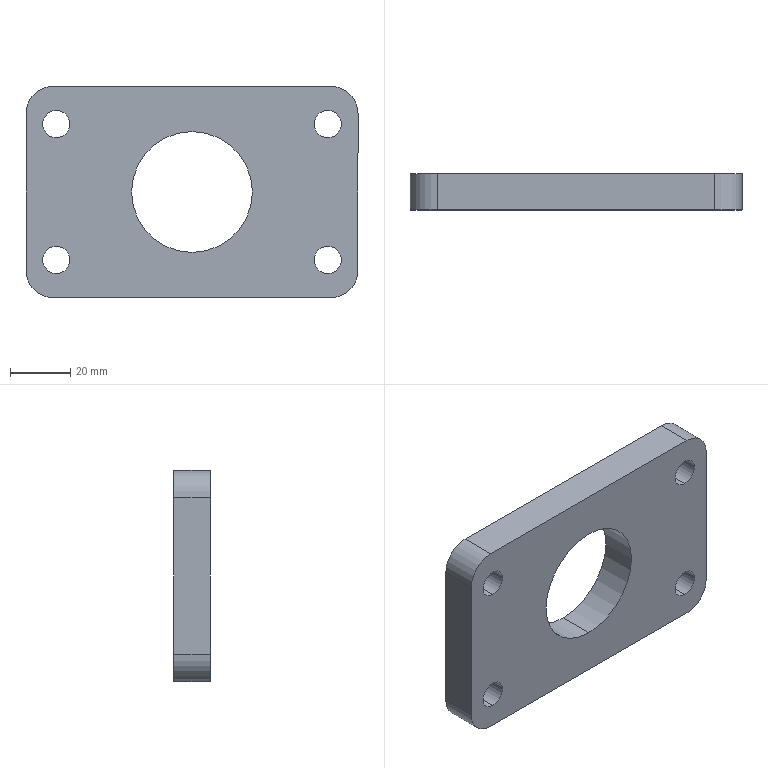Part | SolidWorks | features BaseBody 1 | 1 solid | 20 faces | box 110 x 12 x 70 mm | volume 73432 mm3 | cylinder 14 | plane 6 | commonest cylinder face diameters 9 x8 18 x4 40 x2
STEP:
#1=CARTESIAN_POINT('',(-180.,150.,107.621));
#2=VERTEX_POINT('',#1);
#3=CARTESIAN_POINT('',(-180.,150.,116.621));
#4=VERTEX_POINT('',#3);
#5=CARTESIAN_POINT('',(-180.,150.,112.121));
#6=DIRECTION('',(0.,1.,0.));
#7=DIRECTION('',(0.,0.,1.));
#8=AXIS2_PLACEMENT_3D('',#5,#6,#7);
#9=CIRCLE('',#8,4.5);
#10=EDGE_CURVE('',#2,#4,#9,.T.);
#11=ORIENTED_EDGE('',*,*,#10,.F.);
#12=CARTESIAN_POINT('',(-180.,162.,107.621));
#13=VERTEX_POINT('',#12);
#14=CARTESIAN_POINT('',(-180.,162.,107.621));
#15=DIRECTION('',(0.,1.,0.));
#16=VECTOR('',#15,1000.);
#17=LINE('',#14,#16);
#18=EDGE_CURVE('',#2,#13,#17,.T.);
#19=ORIENTED_EDGE('',*,*,#18,.T.);
#20=CARTESIAN_POINT('',(-180.,162.,116.621));
#21=VERTEX_POINT('',#20);
#22=CARTESIAN_POINT('',(-180.,162.,112.121));
#23=DIRECTION('',(0.,-1.,0.));
#24=DIRECTION('',(0.,0.,1.));
#25=AXIS2_PLACEMENT_3D('',#22,#23,#24);
#26=CIRCLE('',#25,4.5);
#27=EDGE_CURVE('',#21,#13,#26,.T.);
#28=ORIENTED_EDGE('',*,*,#27,.F.);
#29=CARTESIAN_POINT('',(-180.,162.,116.621));
#30=DIRECTION('',(0.,1.,0.));
#31=VECTOR('',#30,1000.);
#32=LINE('',#29,#31);
#33=EDGE_CURVE('',#4,#21,#32,.T.);
#34=ORIENTED_EDGE('',*,*,#33,.F.);
#35=EDGE_LOOP('',(#11,#19,#28,#34));
#36=FACE_OUTER_BOUND('',#35,.T.);
#37=CARTESIAN_POINT('',(-180.,162.,112.121));
#38=DIRECTION('',(0.,1.,0.));
#39=DIRECTION('',(0.,0.,1.));
#40=AXIS2_PLACEMENT_3D('',#37,#38,#39);
#41=CYLINDRICAL_SURFACE('',#40,4.5);
#42=ADVANCED_FACE('',(#36),#41,.F.);
#43=CARTESIAN_POINT('',(-180.,150.,152.621));
#44=VERTEX_POINT('',#43);
#45=CARTESIAN_POINT('',(-180.,150.,161.621));
#46=VERTEX_POINT('',#45);
#47=CARTESIAN_POINT('',(-180.,150.,157.121));
#48=DIRECTION('',(0.,1.,0.));
#49=DIRECTION('',(0.,0.,1.));
#50=AXIS2_PLACEMENT_3D('',#47,#48,#49);
#51=CIRCLE('',#50,4.5);
#52=EDGE_CURVE('',#44,#46,#51,.T.);
#53=ORIENTED_EDGE('',*,*,#52,.F.);
#54=CARTESIAN_POINT('',(-180.,162.,152.621));
#55=VERTEX_POINT('',#54);
#56=CARTESIAN_POINT('',(-180.,162.,152.621));
#57=DIRECTION('',(0.,1.,0.));
#58=VECTOR('',#57,1000.);
#59=LINE('',#56,#58);
#60=EDGE_CURVE('',#44,#55,#59,.T.);
#61=ORIENTED_EDGE('',*,*,#60,.T.);
#62=CARTESIAN_POINT('',(-180.,162.,161.621));
#63=VERTEX_POINT('',#62);
#64=CARTESIAN_POINT('',(-180.,162.,157.121));
#65=DIRECTION('',(0.,-1.,0.));
#66=DIRECTION('',(0.,0.,1.));
#67=AXIS2_PLACEMENT_3D('',#64,#65,#66);
#68=CIRCLE('',#67,4.5);
#69=EDGE_CURVE('',#63,#55,#68,.T.);
#70=ORIENTED_EDGE('',*,*,#69,.F.);
#71=CARTESIAN_POINT('',(-180.,162.,161.621));
#72=DIRECTION('',(0.,1.,0.));
#73=VECTOR('',#72,1000.);
#74=LINE('',#71,#73);
#75=EDGE_CURVE('',#46,#63,#74,.T.);
#76=ORIENTED_EDGE('',*,*,#75,.F.);
#77=EDGE_LOOP('',(#53,#61,#70,#76));
#78=FACE_OUTER_BOUND('',#77,.T.);
#79=CARTESIAN_POINT('',(-180.,162.,157.121));
#80=DIRECTION('',(0.,1.,0.));
#81=DIRECTION('',(0.,0.,1.));
#82=AXIS2_PLACEMENT_3D('',#79,#80,#81);
#83=CYLINDRICAL_SURFACE('',#82,4.5);
#84=ADVANCED_FACE('',(#78),#83,.F.);
#85=CARTESIAN_POINT('',(-225.,150.,114.621));
#86=VERTEX_POINT('',#85);
#87=CARTESIAN_POINT('',(-225.,150.,154.621));
#88=VERTEX_POINT('',#87);
#89=CARTESIAN_POINT('',(-225.,150.,134.621));
#90=DIRECTION('',(0.,1.,0.));
#91=DIRECTION('',(0.,0.,1.));
#92=AXIS2_PLACEMENT_3D('',#89,#90,#91);
#93=CIRCLE('',#92,20.);
#94=EDGE_CURVE('',#86,#88,#93,.T.);
#95=ORIENTED_EDGE('',*,*,#94,.F.);
#96=CARTESIAN_POINT('',(-225.,162.,114.621));
#97=VERTEX_POINT('',#96);
#98=CARTESIAN_POINT('',(-225.,162.,114.621));
#99=DIRECTION('',(0.,1.,0.));
#100=VECTOR('',#99,1000.);
#101=LINE('',#98,#100);
#102=EDGE_CURVE('',#86,#97,#101,.T.);
#103=ORIENTED_EDGE('',*,*,#102,.T.);
#104=CARTESIAN_POINT('',(-225.,162.,154.621));
#105=VERTEX_POINT('',#104);
#106=CARTESIAN_POINT('',(-225.,162.,134.621));
#107=DIRECTION('',(0.,-1.,0.));
#108=DIRECTION('',(0.,0.,1.));
#109=AXIS2_PLACEMENT_3D('',#106,#107,#108);
#110=CIRCLE('',#109,20.);
#111=EDGE_CURVE('',#105,#97,#110,.T.);
#112=ORIENTED_EDGE('',*,*,#111,.F.);
#113=CARTESIAN_POINT('',(-225.,162.,154.621));
#114=DIRECTION('',(0.,1.,0.));
#115=VECTOR('',#114,1000.);
#116=LINE('',#113,#115);
#117=EDGE_CURVE('',#88,#105,#116,.T.);
#118=ORIENTED_EDGE('',*,*,#117,.F.);
#119=EDGE_LOOP('',(#95,#103,#112,#118));
#120=FACE_OUTER_BOUND('',#119,.T.);
#121=CARTESIAN_POINT('',(-225.,162.,134.621));
#122=DIRECTION('',(0.,1.,0.));
#123=DIRECTION('',(0.,0.,1.));
#124=AXIS2_PLACEMENT_3D('',#121,#122,#123);
#125=CYLINDRICAL_SURFACE('',#124,20.);
#126=ADVANCED_FACE('',(#120),#125,.F.);
#127=CARTESIAN_POINT('',(-270.,150.,107.621));
#128=VERTEX_POINT('',#127);
#129=CARTESIAN_POINT('',(-270.,150.,116.621));
#130=VERTEX_POINT('',#129);
#131=CARTESIAN_POINT('',(-270.,150.,112.121));
#132=DIRECTION('',(0.,1.,0.));
#133=DIRECTION('',(0.,0.,1.));
#134=AXIS2_PLACEMENT_3D('',#131,#132,#133);
#135=CIRCLE('',#134,4.5);
#136=EDGE_CURVE('',#128,#130,#135,.T.);
#137=ORIENTED_EDGE('',*,*,#136,.F.);
#138=CARTESIAN_POINT('',(-270.,162.,107.621));
#139=VERTEX_POINT('',#138);
#140=CARTESIAN_POINT('',(-270.,162.,107.621));
#141=DIRECTION('',(0.,1.,0.));
#142=VECTOR('',#141,1000.);
#143=LINE('',#140,#142);
#144=EDGE_CURVE('',#128,#139,#143,.T.);
#145=ORIENTED_EDGE('',*,*,#144,.T.);
#146=CARTESIAN_POINT('',(-270.,162.,116.621));
#147=VERTEX_POINT('',#146);
#148=CARTESIAN_POINT('',(-270.,162.,112.121));
#149=DIRECTION('',(0.,-1.,0.));
#150=DIRECTION('',(0.,0.,1.));
#151=AXIS2_PLACEMENT_3D('',#148,#149,#150);
#152=CIRCLE('',#151,4.5);
#153=EDGE_CURVE('',#147,#139,#152,.T.);
#154=ORIENTED_EDGE('',*,*,#153,.F.);
#155=CARTESIAN_POINT('',(-270.,162.,116.621));
#156=DIRECTION('',(0.,1.,0.));
#157=VECTOR('',#156,1000.);
#158=LINE('',#155,#157);
#159=EDGE_CURVE('',#130,#147,#158,.T.);
#160=ORIENTED_EDGE('',*,*,#159,.F.);
#161=EDGE_LOOP('',(#137,#145,#154,#160));
#162=FACE_OUTER_BOUND('',#161,.T.);
#163=CARTESIAN_POINT('',(-270.,162.,112.121));
#164=DIRECTION('',(0.,1.,0.));
#165=DIRECTION('',(0.,0.,1.));
#166=AXIS2_PLACEMENT_3D('',#163,#164,#165);
#167=CYLINDRICAL_SURFACE('',#166,4.5);
#168=ADVANCED_FACE('',(#162),#167,.F.);
#169=CARTESIAN_POINT('',(-270.,150.,152.621));
#170=VERTEX_POINT('',#169);
#171=CARTESIAN_POINT('',(-270.,150.,161.621));
#172=VERTEX_POINT('',#171);
#173=CARTESIAN_POINT('',(-270.,150.,157.121));
#174=DIRECTION('',(0.,1.,0.));
#175=DIRECTION('',(0.,0.,1.));
#176=AXIS2_PLACEMENT_3D('',#173,#174,#175);
#177=CIRCLE('',#176,4.5);
#178=EDGE_CURVE('',#170,#172,#177,.T.);
#179=ORIENTED_EDGE('',*,*,#178,.F.);
#180=CARTESIAN_POINT('',(-270.,162.,152.621));
#181=VERTEX_POINT('',#180);
#182=CARTESIAN_POINT('',(-270.,162.,152.621));
#183=DIRECTION('',(0.,1.,0.));
#184=VECTOR('',#183,1000.);
#185=LINE('',#182,#184);
#186=EDGE_CURVE('',#170,#181,#185,.T.);
#187=ORIENTED_EDGE('',*,*,#186,.T.);
#188=CARTESIAN_POINT('',(-270.,162.,161.621));
#189=VERTEX_POINT('',#188);
#190=CARTESIAN_POINT('',(-270.,162.,157.121));
#191=DIRECTION('',(0.,-1.,0.));
#192=DIRECTION('',(0.,0.,1.));
#193=AXIS2_PLACEMENT_3D('',#190,#191,#192);
#194=CIRCLE('',#193,4.5);
#195=EDGE_CURVE('',#189,#181,#194,.T.);
#196=ORIENTED_EDGE('',*,*,#195,.F.);
#197=CARTESIAN_POINT('',(-270.,162.,161.621));
#198=DIRECTION('',(0.,1.,0.));
#199=VECTOR('',#198,1000.);
#200=LINE('',#197,#199);
#201=EDGE_CURVE('',#172,#189,#200,.T.);
#202=ORIENTED_EDGE('',*,*,#201,.F.);
#203=EDGE_LOOP('',(#179,#187,#196,#202));
#204=FACE_OUTER_BOUND('',#203,.T.);
#205=CARTESIAN_POINT('',(-270.,162.,157.121));
#206=DIRECTION('',(0.,1.,0.));
#207=DIRECTION('',(0.,0.,1.));
#208=AXIS2_PLACEMENT_3D('',#205,#206,#207);
#209=CYLINDRICAL_SURFACE('',#208,4.5);
#210=ADVANCED_FACE('',(#204),#209,.F.);
#211=CARTESIAN_POINT('',(-170.,150.,108.621));
#212=VERTEX_POINT('',#211);
#213=CARTESIAN_POINT('',(-170.,150.,160.621));
#214=VERTEX_POINT('',#213);
#215=CARTESIAN_POINT('',(-170.,150.,134.621));
#216=DIRECTION('',(0.,0.,1.));
#217=VECTOR('',#216,1000.);
#218=LINE('',#215,#217);
#219=EDGE_CURVE('',#212,#214,#218,.T.);
#220=ORIENTED_EDGE('',*,*,#219,.T.);
#221=CARTESIAN_POINT('',(-179.,150.,169.621));
#222=VERTEX_POINT('',#221);
#223=CARTESIAN_POINT('',(-179.,150.,160.621));
#224=DIRECTION('',(0.,-1.,0.));
#225=DIRECTION('',(0.,0.,1.));
#226=AXIS2_PLACEMENT_3D('',#223,#224,#225);
#227=CIRCLE('',#226,9.);
#228=EDGE_CURVE('',#214,#222,#227,.T.);
#229=ORIENTED_EDGE('',*,*,#228,.T.);
#230=CARTESIAN_POINT('',(-271.,150.,169.621));
#231=VERTEX_POINT('',#230);
#232=CARTESIAN_POINT('',(-225.,150.,169.621));
#233=DIRECTION('',(-1.,0.,0.));
#234=VECTOR('',#233,1000.);
#235=LINE('',#232,#234);
#236=EDGE_CURVE('',#222,#231,#235,.T.);
#237=ORIENTED_EDGE('',*,*,#236,.T.);
#238=CARTESIAN_POINT('',(-280.,150.,160.621));
#239=VERTEX_POINT('',#238);
#240=CARTESIAN_POINT('',(-271.,150.,160.621));
#241=DIRECTION('',(0.,-1.,0.));
#242=DIRECTION('',(0.,0.,1.));
#243=AXIS2_PLACEMENT_3D('',#240,#241,#242);
#244=CIRCLE('',#243,9.);
#245=EDGE_CURVE('',#231,#239,#244,.T.);
#246=ORIENTED_EDGE('',*,*,#245,.T.);
#247=CARTESIAN_POINT('',(-280.,150.,108.621));
#248=VERTEX_POINT('',#247);
#249=CARTESIAN_POINT('',(-280.,150.,134.621));
#250=DIRECTION('',(0.,0.,-1.));
#251=VECTOR('',#250,1000.);
#252=LINE('',#249,#251);
#253=EDGE_CURVE('',#239,#248,#252,.T.);
#254=ORIENTED_EDGE('',*,*,#253,.T.);
#255=CARTESIAN_POINT('',(-271.,150.,99.621));
#256=VERTEX_POINT('',#255);
#257=CARTESIAN_POINT('',(-271.,150.,108.621));
#258=DIRECTION('',(0.,-1.,0.));
#259=DIRECTION('',(0.,0.,1.));
#260=AXIS2_PLACEMENT_3D('',#257,#258,#259);
#261=CIRCLE('',#260,9.);
#262=EDGE_CURVE('',#248,#256,#261,.T.);
#263=ORIENTED_EDGE('',*,*,#262,.T.);
#264=CARTESIAN_POINT('',(-179.,150.,99.621));
#265=VERTEX_POINT('',#264);
#266=CARTESIAN_POINT('',(-225.,150.,99.621));
#267=DIRECTION('',(1.,0.,0.));
#268=VECTOR('',#267,1000.);
#269=LINE('',#266,#268);
#270=EDGE_CURVE('',#256,#265,#269,.T.);
#271=ORIENTED_EDGE('',*,*,#270,.T.);
#272=CARTESIAN_POINT('',(-179.,150.,108.621));
#273=DIRECTION('',(0.,-1.,0.));
#274=DIRECTION('',(0.,0.,1.));
#275=AXIS2_PLACEMENT_3D('',#272,#273,#274);
#276=CIRCLE('',#275,9.);
#277=EDGE_CURVE('',#265,#212,#276,.T.);
#278=ORIENTED_EDGE('',*,*,#277,.T.);
#279=EDGE_LOOP('',(#220,#229,#237,#246,#254,#263,#271,#278));
#280=FACE_OUTER_BOUND('',#279,.T.);
#281=CARTESIAN_POINT('',(-180.,150.,112.121));
#282=DIRECTION('',(0.,1.,0.));
#283=DIRECTION('',(0.,0.,1.));
#284=AXIS2_PLACEMENT_3D('',#281,#282,#283);
#285=CIRCLE('',#284,4.5);
#286=EDGE_CURVE('',#4,#2,#285,.T.);
#287=ORIENTED_EDGE('',*,*,#286,.T.);
#288=ORIENTED_EDGE('',*,*,#10,.T.);
#289=EDGE_LOOP('',(#287,#288));
#290=FACE_BOUND('',#289,.T.);
#291=CARTESIAN_POINT('',(-180.,150.,157.121));
#292=DIRECTION('',(0.,1.,0.));
#293=DIRECTION('',(0.,0.,1.));
#294=AXIS2_PLACEMENT_3D('',#291,#292,#293);
#295=CIRCLE('',#294,4.5);
#296=EDGE_CURVE('',#46,#44,#295,.T.);
#297=ORIENTED_EDGE('',*,*,#296,.T.);
#298=ORIENTED_EDGE('',*,*,#52,.T.);
#299=EDGE_LOOP('',(#297,#298));
#300=FACE_BOUND('',#299,.T.);
#301=CARTESIAN_POINT('',(-225.,150.,134.621));
#302=DIRECTION('',(0.,1.,0.));
#303=DIRECTION('',(0.,0.,1.));
#304=AXIS2_PLACEMENT_3D('',#301,#302,#303);
#305=CIRCLE('',#304,20.);
#306=EDGE_CURVE('',#88,#86,#305,.T.);
#307=ORIENTED_EDGE('',*,*,#306,.T.);
#308=ORIENTED_EDGE('',*,*,#94,.T.);
#309=EDGE_LOOP('',(#307,#308));
#310=FACE_BOUND('',#309,.T.);
#311=CARTESIAN_POINT('',(-270.,150.,112.121));
#312=DIRECTION('',(0.,1.,0.));
#313=DIRECTION('',(0.,0.,1.));
#314=AXIS2_PLACEMENT_3D('',#311,#312,#313);
#315=CIRCLE('',#314,4.5);
#316=EDGE_CURVE('',#130,#128,#315,.T.);
#317=ORIENTED_EDGE('',*,*,#316,.T.);
#318=ORIENTED_EDGE('',*,*,#136,.T.);
#319=EDGE_LOOP('',(#317,#318));
#320=FACE_BOUND('',#319,.T.);
#321=CARTESIAN_POINT('',(-270.,150.,157.121));
#322=DIRECTION('',(0.,1.,0.));
#323=DIRECTION('',(0.,0.,1.));
#324=AXIS2_PLACEMENT_3D('',#321,#322,#323);
#325=CIRCLE('',#324,4.5);
#326=EDGE_CURVE('',#172,#170,#325,.T.);
#327=ORIENTED_EDGE('',*,*,#326,.T.);
#328=ORIENTED_EDGE('',*,*,#178,.T.);
#329=EDGE_LOOP('',(#327,#328));
#330=FACE_BOUND('',#329,.T.);
#331=CARTESIAN_POINT('',(-225.,150.,134.621));
#332=DIRECTION('',(0.,-1.,0.));
#333=DIRECTION('',(0.,0.,-1.));
#334=AXIS2_PLACEMENT_3D('',#331,#332,#333);
#335=PLANE('',#334);
#336=ADVANCED_FACE('',(#280,#290,#300,#310,#320,#330),#335,.T.);
#337=ORIENTED_EDGE('',*,*,#228,.F.);
#338=CARTESIAN_POINT('',(-170.,162.,160.621));
#339=VERTEX_POINT('',#338);
#340=CARTESIAN_POINT('',(-170.,162.,160.621));
#341=DIRECTION('',(0.,1.,0.));
#342=VECTOR('',#341,1000.);
#343=LINE('',#340,#342);
#344=EDGE_CURVE('',#214,#339,#343,.T.);
#345=ORIENTED_EDGE('',*,*,#344,.T.);
#346=CARTESIAN_POINT('',(-179.,162.,169.621));
#347=VERTEX_POINT('',#346);
#348=CARTESIAN_POINT('',(-179.,162.,160.621));
#349=DIRECTION('',(0.,-1.,0.));
#350=DIRECTION('',(0.,0.,1.));
#351=AXIS2_PLACEMENT_3D('',#348,#349,#350);
#352=CIRCLE('',#351,9.);
#353=EDGE_CURVE('',#339,#347,#352,.T.);
#354=ORIENTED_EDGE('',*,*,#353,.T.);
#355=CARTESIAN_POINT('',(-179.,162.,169.621));
#356=DIRECTION('',(0.,-1.,0.));
#357=VECTOR('',#356,1000.);
#358=LINE('',#355,#357);
#359=EDGE_CURVE('',#347,#222,#358,.T.);
#360=ORIENTED_EDGE('',*,*,#359,.T.);
#361=EDGE_LOOP('',(#337,#345,#354,#360));
#362=FACE_OUTER_BOUND('',#361,.T.);
#363=CARTESIAN_POINT('',(-179.,162.,160.621));
#364=DIRECTION('',(0.,1.,0.));
#365=DIRECTION('',(0.,0.,1.));
#366=AXIS2_PLACEMENT_3D('',#363,#364,#365);
#367=CYLINDRICAL_SURFACE('',#366,9.);
#368=ADVANCED_FACE('',(#362),#367,.T.);
#369=ORIENTED_EDGE('',*,*,#219,.F.);
#370=CARTESIAN_POINT('',(-170.,162.,108.621));
#371=VERTEX_POINT('',#370);
#372=CARTESIAN_POINT('',(-170.,162.,108.621));
#373=DIRECTION('',(0.,1.,0.));
#374=VECTOR('',#373,1000.);
#375=LINE('',#372,#374);
#376=EDGE_CURVE('',#212,#371,#375,.T.);
#377=ORIENTED_EDGE('',*,*,#376,.T.);
#378=CARTESIAN_POINT('',(-170.,162.,160.621));
#379=DIRECTION('',(0.,0.,1.));
#380=VECTOR('',#379,1000.);
#381=LINE('',#378,#380);
#382=EDGE_CURVE('',#371,#339,#381,.T.);
#383=ORIENTED_EDGE('',*,*,#382,.T.);
#384=ORIENTED_EDGE('',*,*,#344,.F.);
#385=EDGE_LOOP('',(#369,#377,#383,#384));
#386=FACE_OUTER_BOUND('',#385,.T.);
#387=CARTESIAN_POINT('',(-170.,162.,160.621));
#388=DIRECTION('',(1.,0.,0.));
#389=DIRECTION('',(0.,0.,-1.));
#390=AXIS2_PLACEMENT_3D('',#387,#388,#389);
#391=PLANE('',#390);
#392=ADVANCED_FACE('',(#386),#391,.T.);
#393=ORIENTED_EDGE('',*,*,#277,.F.);
#394=CARTESIAN_POINT('',(-179.,162.,99.621));
#395=VERTEX_POINT('',#394);
#396=CARTESIAN_POINT('',(-179.,162.,99.621));
#397=DIRECTION('',(0.,1.,0.));
#398=VECTOR('',#397,1000.);
#399=LINE('',#396,#398);
#400=EDGE_CURVE('',#265,#395,#399,.T.);
#401=ORIENTED_EDGE('',*,*,#400,.T.);
#402=CARTESIAN_POINT('',(-179.,162.,108.621));
#403=DIRECTION('',(0.,-1.,0.));
#404=DIRECTION('',(0.,0.,1.));
#405=AXIS2_PLACEMENT_3D('',#402,#403,#404);
#406=CIRCLE('',#405,9.);
#407=EDGE_CURVE('',#395,#371,#406,.T.);
#408=ORIENTED_EDGE('',*,*,#407,.T.);
#409=ORIENTED_EDGE('',*,*,#376,.F.);
#410=EDGE_LOOP('',(#393,#401,#408,#409));
#411=FACE_OUTER_BOUND('',#410,.T.);
#412=CARTESIAN_POINT('',(-179.,162.,108.621));
#413=DIRECTION('',(0.,1.,0.));
#414=DIRECTION('',(0.,0.,1.));
#415=AXIS2_PLACEMENT_3D('',#412,#413,#414);
#416=CYLINDRICAL_SURFACE('',#415,9.);
#417=ADVANCED_FACE('',(#411),#416,.T.);
#418=ORIENTED_EDGE('',*,*,#270,.F.);
#419=CARTESIAN_POINT('',(-271.,162.,99.621));
#420=VERTEX_POINT('',#419);
#421=CARTESIAN_POINT('',(-271.,162.,99.621));
#422=DIRECTION('',(0.,1.,0.));
#423=VECTOR('',#422,1000.);
#424=LINE('',#421,#423);
#425=EDGE_CURVE('',#256,#420,#424,.T.);
#426=ORIENTED_EDGE('',*,*,#425,.T.);
#427=CARTESIAN_POINT('',(-179.,162.,99.621));
#428=DIRECTION('',(1.,0.,0.));
#429=VECTOR('',#428,1000.);
#430=LINE('',#427,#429);
#431=EDGE_CURVE('',#420,#395,#430,.T.);
#432=ORIENTED_EDGE('',*,*,#431,.T.);
#433=ORIENTED_EDGE('',*,*,#400,.F.);
#434=EDGE_LOOP('',(#418,#426,#432,#433));
#435=FACE_OUTER_BOUND('',#434,.T.);
#436=CARTESIAN_POINT('',(-179.,162.,99.621));
#437=DIRECTION('',(0.,0.,-1.));
#438=DIRECTION('',(-1.,0.,0.));
#439=AXIS2_PLACEMENT_3D('',#436,#437,#438);
#440=PLANE('',#439);
#441=ADVANCED_FACE('',(#435),#440,.T.);
#442=ORIENTED_EDGE('',*,*,#262,.F.);
#443=CARTESIAN_POINT('',(-280.,162.,108.621));
#444=VERTEX_POINT('',#443);
#445=CARTESIAN_POINT('',(-280.,162.,108.621));
#446=DIRECTION('',(0.,1.,0.));
#447=VECTOR('',#446,1000.);
#448=LINE('',#445,#447);
#449=EDGE_CURVE('',#248,#444,#448,.T.);
#450=ORIENTED_EDGE('',*,*,#449,.T.);
#451=CARTESIAN_POINT('',(-271.,162.,108.621));
#452=DIRECTION('',(0.,-1.,0.));
#453=DIRECTION('',(0.,0.,1.));
#454=AXIS2_PLACEMENT_3D('',#451,#452,#453);
#455=CIRCLE('',#454,9.);
#456=EDGE_CURVE('',#444,#420,#455,.T.);
#457=ORIENTED_EDGE('',*,*,#456,.T.);
#458=ORIENTED_EDGE('',*,*,#425,.F.);
#459=EDGE_LOOP('',(#442,#450,#457,#458));
#460=FACE_OUTER_BOUND('',#459,.T.);
#461=CARTESIAN_POINT('',(-271.,162.,108.621));
#462=DIRECTION('',(0.,1.,0.));
#463=DIRECTION('',(0.,0.,1.));
#464=AXIS2_PLACEMENT_3D('',#461,#462,#463);
#465=CYLINDRICAL_SURFACE('',#464,9.);
#466=ADVANCED_FACE('',(#460),#465,.T.);
#467=ORIENTED_EDGE('',*,*,#253,.F.);
#468=CARTESIAN_POINT('',(-280.,162.,160.621));
#469=VERTEX_POINT('',#468);
#470=CARTESIAN_POINT('',(-280.,162.,160.621));
#471=DIRECTION('',(0.,1.,0.));
#472=VECTOR('',#471,1000.);
#473=LINE('',#470,#472);
#474=EDGE_CURVE('',#239,#469,#473,.T.);
#475=ORIENTED_EDGE('',*,*,#474,.T.);
#476=CARTESIAN_POINT('',(-280.,162.,108.621));
#477=DIRECTION('',(0.,0.,-1.));
#478=VECTOR('',#477,1000.);
#479=LINE('',#476,#478);
#480=EDGE_CURVE('',#469,#444,#479,.T.);
#481=ORIENTED_EDGE('',*,*,#480,.T.);
#482=ORIENTED_EDGE('',*,*,#449,.F.);
#483=EDGE_LOOP('',(#467,#475,#481,#482));
#484=FACE_OUTER_BOUND('',#483,.T.);
#485=CARTESIAN_POINT('',(-280.,162.,108.621));
#486=DIRECTION('',(-1.,0.,0.));
#487=DIRECTION('',(0.,0.,1.));
#488=AXIS2_PLACEMENT_3D('',#485,#486,#487);
#489=PLANE('',#488);
#490=ADVANCED_FACE('',(#484),#489,.T.);
#491=ORIENTED_EDGE('',*,*,#245,.F.);
#492=CARTESIAN_POINT('',(-271.,162.,169.621));
#493=VERTEX_POINT('',#492);
#494=CARTESIAN_POINT('',(-271.,162.,169.621));
#495=DIRECTION('',(0.,1.,0.));
#496=VECTOR('',#495,1000.);
#497=LINE('',#494,#496);
#498=EDGE_CURVE('',#231,#493,#497,.T.);
#499=ORIENTED_EDGE('',*,*,#498,.T.);
#500=CARTESIAN_POINT('',(-271.,162.,160.621));
#501=DIRECTION('',(0.,-1.,0.));
#502=DIRECTION('',(0.,0.,1.));
#503=AXIS2_PLACEMENT_3D('',#500,#501,#502);
#504=CIRCLE('',#503,9.);
#505=EDGE_CURVE('',#493,#469,#504,.T.);
#506=ORIENTED_EDGE('',*,*,#505,.T.);
#507=ORIENTED_EDGE('',*,*,#474,.F.);
#508=EDGE_LOOP('',(#491,#499,#506,#507));
#509=FACE_OUTER_BOUND('',#508,.T.);
#510=CARTESIAN_POINT('',(-271.,162.,160.621));
#511=DIRECTION('',(0.,1.,0.));
#512=DIRECTION('',(0.,0.,1.));
#513=AXIS2_PLACEMENT_3D('',#510,#511,#512);
#514=CYLINDRICAL_SURFACE('',#513,9.);
#515=ADVANCED_FACE('',(#509),#514,.T.);
#516=ORIENTED_EDGE('',*,*,#236,.F.);
#517=ORIENTED_EDGE('',*,*,#359,.F.);
#518=CARTESIAN_POINT('',(-271.,162.,169.621));
#519=DIRECTION('',(-1.,0.,0.));
#520=VECTOR('',#519,1000.);
#521=LINE('',#518,#520);
#522=EDGE_CURVE('',#347,#493,#521,.T.);
#523=ORIENTED_EDGE('',*,*,#522,.T.);
#524=ORIENTED_EDGE('',*,*,#498,.F.);
#525=EDGE_LOOP('',(#516,#517,#523,#524));
#526=FACE_OUTER_BOUND('',#525,.T.);
#527=CARTESIAN_POINT('',(-271.,162.,169.621));
#528=DIRECTION('',(0.,0.,1.));
#529=DIRECTION('',(1.,0.,0.));
#530=AXIS2_PLACEMENT_3D('',#527,#528,#529);
#531=PLANE('',#530);
#532=ADVANCED_FACE('',(#526),#531,.T.);
#533=ORIENTED_EDGE('',*,*,#18,.F.);
#534=ORIENTED_EDGE('',*,*,#286,.F.);
#535=ORIENTED_EDGE('',*,*,#33,.T.);
#536=CARTESIAN_POINT('',(-180.,162.,112.121));
#537=DIRECTION('',(0.,-1.,0.));
#538=DIRECTION('',(0.,0.,1.));
#539=AXIS2_PLACEMENT_3D('',#536,#537,#538);
#540=CIRCLE('',#539,4.5);
#541=EDGE_CURVE('',#13,#21,#540,.T.);
#542=ORIENTED_EDGE('',*,*,#541,.F.);
#543=EDGE_LOOP('',(#533,#534,#535,#542));
#544=FACE_OUTER_BOUND('',#543,.T.);
#545=CARTESIAN_POINT('',(-180.,162.,112.121));
#546=DIRECTION('',(0.,1.,0.));
#547=DIRECTION('',(0.,0.,1.));
#548=AXIS2_PLACEMENT_3D('',#545,#546,#547);
#549=CYLINDRICAL_SURFACE('',#548,4.5);
#550=ADVANCED_FACE('',(#544),#549,.F.);
#551=ORIENTED_EDGE('',*,*,#60,.F.);
#552=ORIENTED_EDGE('',*,*,#296,.F.);
#553=ORIENTED_EDGE('',*,*,#75,.T.);
#554=CARTESIAN_POINT('',(-180.,162.,157.121));
#555=DIRECTION('',(0.,-1.,0.));
#556=DIRECTION('',(0.,0.,1.));
#557=AXIS2_PLACEMENT_3D('',#554,#555,#556);
#558=CIRCLE('',#557,4.5);
#559=EDGE_CURVE('',#55,#63,#558,.T.);
#560=ORIENTED_EDGE('',*,*,#559,.F.);
#561=EDGE_LOOP('',(#551,#552,#553,#560));
#562=FACE_OUTER_BOUND('',#561,.T.);
#563=CARTESIAN_POINT('',(-180.,162.,157.121));
#564=DIRECTION('',(0.,1.,0.));
#565=DIRECTION('',(0.,0.,1.));
#566=AXIS2_PLACEMENT_3D('',#563,#564,#565);
#567=CYLINDRICAL_SURFACE('',#566,4.5);
#568=ADVANCED_FACE('',(#562),#567,.F.);
#569=ORIENTED_EDGE('',*,*,#102,.F.);
#570=ORIENTED_EDGE('',*,*,#306,.F.);
#571=ORIENTED_EDGE('',*,*,#117,.T.);
#572=CARTESIAN_POINT('',(-225.,162.,134.621));
#573=DIRECTION('',(0.,-1.,0.));
#574=DIRECTION('',(0.,0.,1.));
#575=AXIS2_PLACEMENT_3D('',#572,#573,#574);
#576=CIRCLE('',#575,20.);
#577=EDGE_CURVE('',#97,#105,#576,.T.);
#578=ORIENTED_EDGE('',*,*,#577,.F.);
#579=EDGE_LOOP('',(#569,#570,#571,#578));
#580=FACE_OUTER_BOUND('',#579,.T.);
#581=CARTESIAN_POINT('',(-225.,162.,134.621));
#582=DIRECTION('',(0.,1.,0.));
#583=DIRECTION('',(0.,0.,1.));
#584=AXIS2_PLACEMENT_3D('',#581,#582,#583);
#585=CYLINDRICAL_SURFACE('',#584,20.);
#586=ADVANCED_FACE('',(#580),#585,.F.);
#587=ORIENTED_EDGE('',*,*,#144,.F.);
#588=ORIENTED_EDGE('',*,*,#316,.F.);
#589=ORIENTED_EDGE('',*,*,#159,.T.);
#590=CARTESIAN_POINT('',(-270.,162.,112.121));
#591=DIRECTION('',(0.,-1.,0.));
#592=DIRECTION('',(0.,0.,1.));
#593=AXIS2_PLACEMENT_3D('',#590,#591,#592);
#594=CIRCLE('',#593,4.5);
#595=EDGE_CURVE('',#139,#147,#594,.T.);
#596=ORIENTED_EDGE('',*,*,#595,.F.);
#597=EDGE_LOOP('',(#587,#588,#589,#596));
#598=FACE_OUTER_BOUND('',#597,.T.);
#599=CARTESIAN_POINT('',(-270.,162.,112.121));
#600=DIRECTION('',(0.,1.,0.));
#601=DIRECTION('',(0.,0.,1.));
#602=AXIS2_PLACEMENT_3D('',#599,#600,#601);
#603=CYLINDRICAL_SURFACE('',#602,4.5);
#604=ADVANCED_FACE('',(#598),#603,.F.);
#605=ORIENTED_EDGE('',*,*,#186,.F.);
#606=ORIENTED_EDGE('',*,*,#326,.F.);
#607=ORIENTED_EDGE('',*,*,#201,.T.);
#608=CARTESIAN_POINT('',(-270.,162.,157.121));
#609=DIRECTION('',(0.,-1.,0.));
#610=DIRECTION('',(0.,0.,1.));
#611=AXIS2_PLACEMENT_3D('',#608,#609,#610);
#612=CIRCLE('',#611,4.5);
#613=EDGE_CURVE('',#181,#189,#612,.T.);
#614=ORIENTED_EDGE('',*,*,#613,.F.);
#615=EDGE_LOOP('',(#605,#606,#607,#614));
#616=FACE_OUTER_BOUND('',#615,.T.);
#617=CARTESIAN_POINT('',(-270.,162.,157.121));
#618=DIRECTION('',(0.,1.,0.));
#619=DIRECTION('',(0.,0.,1.));
#620=AXIS2_PLACEMENT_3D('',#617,#618,#619);
#621=CYLINDRICAL_SURFACE('',#620,4.5);
#622=ADVANCED_FACE('',(#616),#621,.F.);
#623=ORIENTED_EDGE('',*,*,#505,.F.);
#624=ORIENTED_EDGE('',*,*,#522,.F.);
#625=ORIENTED_EDGE('',*,*,#353,.F.);
#626=ORIENTED_EDGE('',*,*,#382,.F.);
#627=ORIENTED_EDGE('',*,*,#407,.F.);
#628=ORIENTED_EDGE('',*,*,#431,.F.);
#629=ORIENTED_EDGE('',*,*,#456,.F.);
#630=ORIENTED_EDGE('',*,*,#480,.F.);
#631=EDGE_LOOP('',(#623,#624,#625,#626,#627,#628,#629,#630));
#632=FACE_OUTER_BOUND('',#631,.T.);
#633=ORIENTED_EDGE('',*,*,#27,.T.);
#634=ORIENTED_EDGE('',*,*,#541,.T.);
#635=EDGE_LOOP('',(#633,#634));
#636=FACE_BOUND('',#635,.T.);
#637=ORIENTED_EDGE('',*,*,#69,.T.);
#638=ORIENTED_EDGE('',*,*,#559,.T.);
#639=EDGE_LOOP('',(#637,#638));
#640=FACE_BOUND('',#639,.T.);
#641=ORIENTED_EDGE('',*,*,#111,.T.);
#642=ORIENTED_EDGE('',*,*,#577,.T.);
#643=EDGE_LOOP('',(#641,#642));
#644=FACE_BOUND('',#643,.T.);
#645=ORIENTED_EDGE('',*,*,#153,.T.);
#646=ORIENTED_EDGE('',*,*,#595,.T.);
#647=EDGE_LOOP('',(#645,#646));
#648=FACE_BOUND('',#647,.T.);
#649=ORIENTED_EDGE('',*,*,#195,.T.);
#650=ORIENTED_EDGE('',*,*,#613,.T.);
#651=EDGE_LOOP('',(#649,#650));
#652=FACE_BOUND('',#651,.T.);
#653=CARTESIAN_POINT('',(-225.,162.,134.621));
#654=DIRECTION('',(0.,-1.,0.));
#655=DIRECTION('',(0.,0.,-1.));
#656=AXIS2_PLACEMENT_3D('',#653,#654,#655);
#657=PLANE('',#656);
#658=ADVANCED_FACE('',(#632,#636,#640,#644,#648,#652),#657,.F.);
#659=CLOSED_SHELL('',(#42,#84,#126,#168,#210,#336,#368,#392,#417,#441,#466,#490,#515,#532,#550,#568,#586,#604,#622,#658));
#660=MANIFOLD_SOLID_BREP('',#659);
#661=CARTESIAN_POINT('',(0.,0.,0.));
#662=DIRECTION('',(0.,0.,1.));
#663=DIRECTION('',(1.,0.,0.));
#664=AXIS2_PLACEMENT_3D('',#661,#662,#663);
#665=(LENGTH_UNIT()NAMED_UNIT(*)SI_UNIT(.MILLI.,.METRE.));
#666=UNCERTAINTY_MEASURE_WITH_UNIT(LENGTH_MEASURE(0.00001),#665,'','');
#667=(NAMED_UNIT(*)PLANE_ANGLE_UNIT()SI_UNIT($,.RADIAN.));
#668=(NAMED_UNIT(*)SI_UNIT($,.STERADIAN.)SOLID_ANGLE_UNIT());
#669=(GEOMETRIC_REPRESENTATION_CONTEXT(3)GLOBAL_UNCERTAINTY_ASSIGNED_CONTEXT((#666))GLOBAL_UNIT_ASSIGNED_CONTEXT((#665,#667,#668))REPRESENTATION_CONTEXT('',''));
#670=ADVANCED_BREP_SHAPE_REPRESENTATION('',(#660,#664),#669);